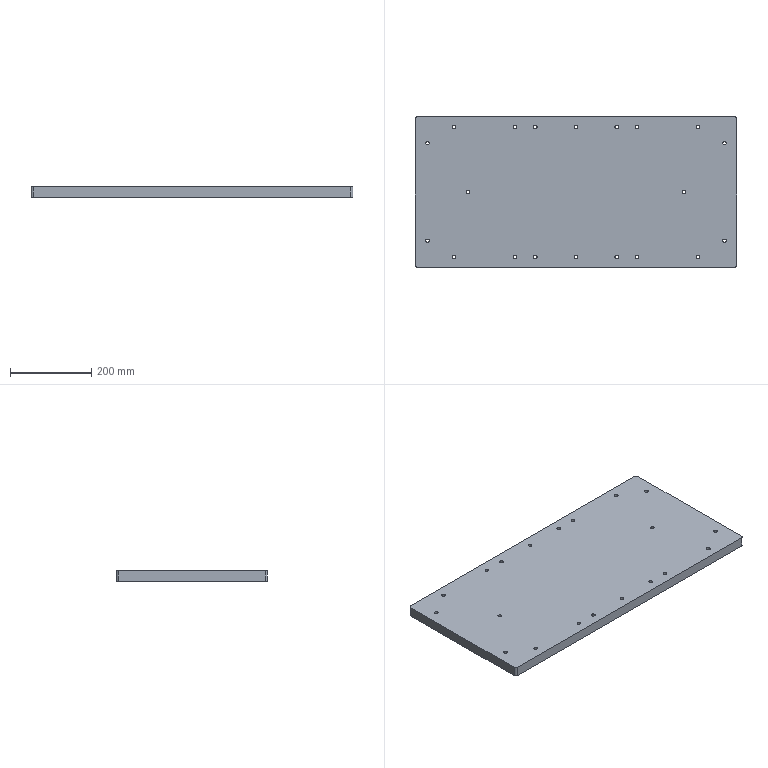Part | 1 solid | 74 faces | box 790 x 370 x 25 mm | volume 7102430 mm3 | cylinder 60 | plane 14 | commonest cylinder face diameters 8.7 x24 9 x16 10 x16 10.5 x4